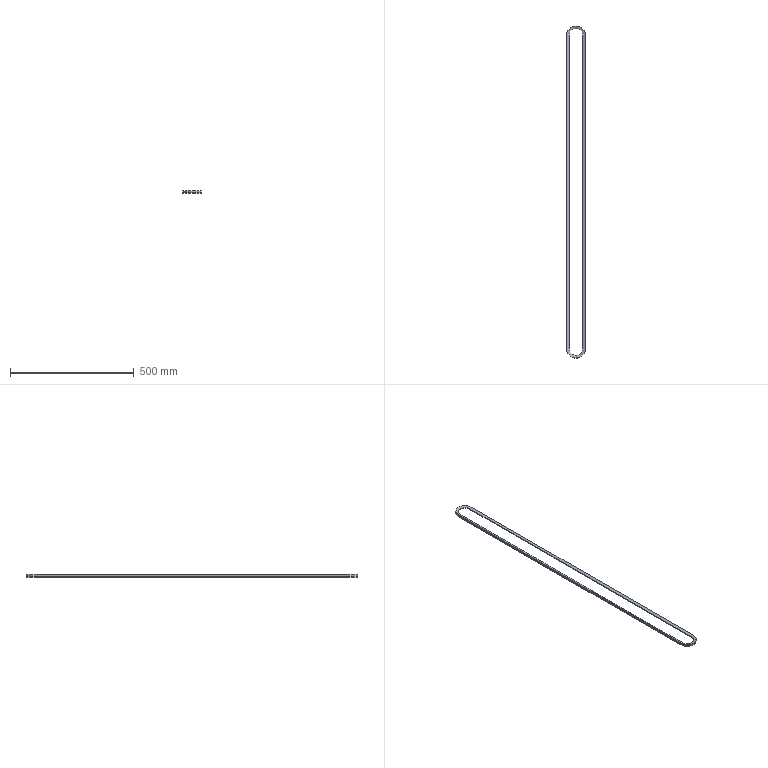Part | STEP file | 103000006124 | 1 solid | 24 faces | box 75 x 1341 x 10 mm | volume 174412 mm3 | plane 12 | cylinder 8 | cone 4 | commonest cylinder face diameters 55 x4 75 x4
STEP:
#1=CARTESIAN_POINT('',(27.5,-1266.,-1.36));
#2=VERTEX_POINT('',#1);
#3=CARTESIAN_POINT('',(37.5,-1266.,-5.));
#4=VERTEX_POINT('',#3);
#5=CARTESIAN_POINT('',(32.5,-1266.,-3.18));
#6=DIRECTION('',(0.9397,0.,-0.342));
#7=VECTOR('',#6,1.);
#8=LINE('',#5,#7);
#9=EDGE_CURVE('',#2,#4,#8,.T.);
#10=ORIENTED_EDGE('',*,*,#9,.F.);
#11=CARTESIAN_POINT('',(27.5,0.,-1.36));
#12=VERTEX_POINT('',#11);
#13=CARTESIAN_POINT('',(27.5,-633.,-1.36));
#14=DIRECTION('',(0.,1.,0.));
#15=VECTOR('',#14,1.);
#16=LINE('',#13,#15);
#17=EDGE_CURVE('',#2,#12,#16,.T.);
#18=ORIENTED_EDGE('',*,*,#17,.T.);
#19=CARTESIAN_POINT('',(37.5,0.,-5.));
#20=VERTEX_POINT('',#19);
#21=CARTESIAN_POINT('',(32.5,0.,-3.18));
#22=DIRECTION('',(0.9397,0.,-0.342));
#23=VECTOR('',#22,1.);
#24=LINE('',#21,#23);
#25=EDGE_CURVE('',#12,#20,#24,.T.);
#26=ORIENTED_EDGE('',*,*,#25,.T.);
#27=CARTESIAN_POINT('',(37.5,-633.,-5.));
#28=DIRECTION('',(0.,1.,0.));
#29=VECTOR('',#28,1.);
#30=LINE('',#27,#29);
#31=EDGE_CURVE('',#4,#20,#30,.T.);
#32=ORIENTED_EDGE('',*,*,#31,.F.);
#33=EDGE_LOOP('',(#10,#18,#26,#32));
#34=FACE_OUTER_BOUND('',#33,.T.);
#35=CARTESIAN_POINT('',(37.5,-1266.,-5.));
#36=DIRECTION('',(0.342,0.,0.9397));
#37=DIRECTION('',(0.9397,0.,-0.342));
#38=AXIS2_PLACEMENT_3D('',#35,#36,#37);
#39=PLANE('',#38);
#40=ADVANCED_FACE('',(#34),#39,.F.);
#41=CARTESIAN_POINT('',(-37.5,-1266.,-5.));
#42=VERTEX_POINT('',#41);
#43=CARTESIAN_POINT('',(0.,-1266.,-5.));
#44=DIRECTION('',(0.,0.,-1.));
#45=AXIS2_PLACEMENT_3D('',#43,#44,$);
#46=CIRCLE('',#45,37.5);
#47=EDGE_CURVE('',#42,#4,#46,.F.);
#48=ORIENTED_EDGE('',*,*,#47,.F.);
#49=CARTESIAN_POINT('',(-27.5,-1266.,-1.36));
#50=VERTEX_POINT('',#49);
#51=CARTESIAN_POINT('',(-469860.06,-1266.,-171006.427));
#52=DIRECTION('',(-0.9397,0.,-0.342));
#53=VECTOR('',#52,1.);
#54=LINE('',#51,#53);
#55=EDGE_CURVE('',#50,#42,#54,.T.);
#56=ORIENTED_EDGE('',*,*,#55,.F.);
#57=CARTESIAN_POINT('',(0.,-1266.,-1.36));
#58=DIRECTION('',(0.,0.,-1.));
#59=AXIS2_PLACEMENT_3D('',#57,#58,$);
#60=CIRCLE('',#59,27.5);
#61=EDGE_CURVE('',#50,#2,#60,.F.);
#62=ORIENTED_EDGE('',*,*,#61,.T.);
#63=ORIENTED_EDGE('',*,*,#9,.T.);
#64=EDGE_LOOP('',(#48,#56,#62,#63));
#65=FACE_OUTER_BOUND('',#64,.T.);
#66=CARTESIAN_POINT('',(0.,-1266.,-1.36));
#67=DIRECTION('',(0.,0.,-1.));
#68=DIRECTION('',(1.,0.,0.));
#69=AXIS2_PLACEMENT_3D('',#66,#67,#68);
#70=CONICAL_SURFACE('',#69,27.5,1.222);
#71=ADVANCED_FACE('',(#65),#70,.F.);
#72=CARTESIAN_POINT('',(27.5,-1266.,0.));
#73=VERTEX_POINT('',#72);
#74=CARTESIAN_POINT('',(27.5,0.,0.));
#75=VERTEX_POINT('',#74);
#76=CARTESIAN_POINT('',(27.5,-633.,0.));
#77=DIRECTION('',(0.,1.,0.));
#78=VECTOR('',#77,1.);
#79=LINE('',#76,#78);
#80=EDGE_CURVE('',#73,#75,#79,.T.);
#81=ORIENTED_EDGE('',*,*,#80,.T.);
#82=CARTESIAN_POINT('',(27.5,0.,-0.6801));
#83=DIRECTION('',(0.,0.,-1.));
#84=VECTOR('',#83,1.);
#85=LINE('',#82,#84);
#86=EDGE_CURVE('',#75,#12,#85,.T.);
#87=ORIENTED_EDGE('',*,*,#86,.T.);
#88=ORIENTED_EDGE('',*,*,#17,.F.);
#89=CARTESIAN_POINT('',(27.5,-1266.,-0.6801));
#90=DIRECTION('',(0.,0.,-1.));
#91=VECTOR('',#90,1.);
#92=LINE('',#89,#91);
#93=EDGE_CURVE('',#73,#2,#92,.T.);
#94=ORIENTED_EDGE('',*,*,#93,.F.);
#95=EDGE_LOOP('',(#81,#87,#88,#94));
#96=FACE_OUTER_BOUND('',#95,.T.);
#97=CARTESIAN_POINT('',(27.5,-1266.,0.));
#98=DIRECTION('',(1.,0.,0.));
#99=DIRECTION('',(0.,1.,0.));
#100=AXIS2_PLACEMENT_3D('',#97,#98,#99);
#101=PLANE('',#100);
#102=ADVANCED_FACE('',(#96),#101,.F.);
#103=CARTESIAN_POINT('',(-37.5,0.,-5.));
#104=VERTEX_POINT('',#103);
#105=CARTESIAN_POINT('',(0.,0.,-5.));
#106=DIRECTION('',(0.,0.,-1.));
#107=AXIS2_PLACEMENT_3D('',#105,#106,$);
#108=CIRCLE('',#107,37.5);
#109=EDGE_CURVE('',#20,#104,#108,.F.);
#110=ORIENTED_EDGE('',*,*,#109,.F.);
#111=ORIENTED_EDGE('',*,*,#25,.F.);
#112=CARTESIAN_POINT('',(-27.5,0.,-1.36));
#113=VERTEX_POINT('',#112);
#114=CARTESIAN_POINT('',(0.,0.,-1.36));
#115=DIRECTION('',(0.,0.,-1.));
#116=AXIS2_PLACEMENT_3D('',#114,#115,$);
#117=CIRCLE('',#116,27.5);
#118=EDGE_CURVE('',#12,#113,#117,.F.);
#119=ORIENTED_EDGE('',*,*,#118,.T.);
#120=CARTESIAN_POINT('',(-469860.06,0.,-171006.427));
#121=DIRECTION('',(-0.9397,0.,-0.342));
#122=VECTOR('',#121,1.);
#123=LINE('',#120,#122);
#124=EDGE_CURVE('',#113,#104,#123,.T.);
#125=ORIENTED_EDGE('',*,*,#124,.T.);
#126=EDGE_LOOP('',(#110,#111,#119,#125));
#127=FACE_OUTER_BOUND('',#126,.T.);
#128=CARTESIAN_POINT('',(0.,0.,-1.36));
#129=DIRECTION('',(0.,0.,-1.));
#130=DIRECTION('',(-1.,0.,0.));
#131=AXIS2_PLACEMENT_3D('',#128,#129,#130);
#132=CONICAL_SURFACE('',#131,27.5,1.222);
#133=ADVANCED_FACE('',(#127),#132,.F.);
#134=ORIENTED_EDGE('',*,*,#31,.T.);
#135=CARTESIAN_POINT('',(37.5,0.,0.));
#136=VERTEX_POINT('',#135);
#137=CARTESIAN_POINT('',(37.5,0.,-2.5));
#138=DIRECTION('',(0.,0.,1.));
#139=VECTOR('',#138,1.);
#140=LINE('',#137,#139);
#141=EDGE_CURVE('',#20,#136,#140,.T.);
#142=ORIENTED_EDGE('',*,*,#141,.T.);
#143=CARTESIAN_POINT('',(37.5,-1266.,0.));
#144=VERTEX_POINT('',#143);
#145=CARTESIAN_POINT('',(37.5,-633.,0.));
#146=DIRECTION('',(0.,1.,0.));
#147=VECTOR('',#146,1.);
#148=LINE('',#145,#147);
#149=EDGE_CURVE('',#144,#136,#148,.T.);
#150=ORIENTED_EDGE('',*,*,#149,.F.);
#151=CARTESIAN_POINT('',(37.5,-1266.,-2.5));
#152=DIRECTION('',(0.,0.,1.));
#153=VECTOR('',#152,1.);
#154=LINE('',#151,#153);
#155=EDGE_CURVE('',#4,#144,#154,.T.);
#156=ORIENTED_EDGE('',*,*,#155,.F.);
#157=EDGE_LOOP('',(#134,#142,#150,#156));
#158=FACE_OUTER_BOUND('',#157,.T.);
#159=CARTESIAN_POINT('',(37.5,-1266.,0.));
#160=DIRECTION('',(-1.,0.,0.));
#161=DIRECTION('',(0.,-1.,0.));
#162=AXIS2_PLACEMENT_3D('',#159,#160,#161);
#163=PLANE('',#162);
#164=ADVANCED_FACE('',(#158),#163,.F.);
#165=CARTESIAN_POINT('',(-37.5,-1266.,0.));
#166=VERTEX_POINT('',#165);
#167=CARTESIAN_POINT('',(0.,-1266.,0.));
#168=DIRECTION('',(0.,0.,1.));
#169=AXIS2_PLACEMENT_3D('',#167,#168,$);
#170=CIRCLE('',#169,37.5);
#171=EDGE_CURVE('',#166,#144,#170,.T.);
#172=ORIENTED_EDGE('',*,*,#171,.F.);
#173=CARTESIAN_POINT('',(-37.5,-1266.,0.));
#174=DIRECTION('',(0.,0.,1.));
#175=VECTOR('',#174,1.);
#176=LINE('',#173,#175);
#177=EDGE_CURVE('',#42,#166,#176,.T.);
#178=ORIENTED_EDGE('',*,*,#177,.F.);
#179=ORIENTED_EDGE('',*,*,#47,.T.);
#180=ORIENTED_EDGE('',*,*,#155,.T.);
#181=EDGE_LOOP('',(#172,#178,#179,#180));
#182=FACE_OUTER_BOUND('',#181,.T.);
#183=CARTESIAN_POINT('',(0.,-1266.,0.));
#184=DIRECTION('',(0.,0.,1.));
#185=DIRECTION('',(-1.,0.,0.));
#186=AXIS2_PLACEMENT_3D('',#183,#184,#185);
#187=CYLINDRICAL_SURFACE('',#186,37.5);
#188=ADVANCED_FACE('',(#182),#187,.T.);
#189=CARTESIAN_POINT('',(-37.5,-633.,-5.));
#190=DIRECTION('',(0.,-1.,0.));
#191=VECTOR('',#190,1.);
#192=LINE('',#189,#191);
#193=EDGE_CURVE('',#104,#42,#192,.T.);
#194=ORIENTED_EDGE('',*,*,#193,.F.);
#195=ORIENTED_EDGE('',*,*,#124,.F.);
#196=CARTESIAN_POINT('',(-27.5,-633.,-1.36));
#197=DIRECTION('',(0.,-1.,0.));
#198=VECTOR('',#197,1.);
#199=LINE('',#196,#198);
#200=EDGE_CURVE('',#113,#50,#199,.T.);
#201=ORIENTED_EDGE('',*,*,#200,.T.);
#202=ORIENTED_EDGE('',*,*,#55,.T.);
#203=EDGE_LOOP('',(#194,#195,#201,#202));
#204=FACE_OUTER_BOUND('',#203,.T.);
#205=CARTESIAN_POINT('',(-37.5,0.,-5.));
#206=DIRECTION('',(-0.342,0.,0.9397));
#207=DIRECTION('',(0.9397,0.,0.342));
#208=AXIS2_PLACEMENT_3D('',#205,#206,#207);
#209=PLANE('',#208);
#210=ADVANCED_FACE('',(#204),#209,.F.);
#211=ORIENTED_EDGE('',*,*,#93,.T.);
#212=ORIENTED_EDGE('',*,*,#61,.F.);
#213=CARTESIAN_POINT('',(-27.5,-1266.,0.));
#214=VERTEX_POINT('',#213);
#215=CARTESIAN_POINT('',(-27.5,-1266.,0.));
#216=DIRECTION('',(0.,0.,1.));
#217=VECTOR('',#216,1.);
#218=LINE('',#215,#217);
#219=EDGE_CURVE('',#214,#50,#218,.F.);
#220=ORIENTED_EDGE('',*,*,#219,.F.);
#221=CARTESIAN_POINT('',(0.,-1266.,0.));
#222=DIRECTION('',(0.,0.,1.));
#223=AXIS2_PLACEMENT_3D('',#221,#222,$);
#224=CIRCLE('',#223,27.5);
#225=EDGE_CURVE('',#214,#73,#224,.T.);
#226=ORIENTED_EDGE('',*,*,#225,.T.);
#227=EDGE_LOOP('',(#211,#212,#220,#226));
#228=FACE_OUTER_BOUND('',#227,.T.);
#229=CARTESIAN_POINT('',(0.,-1266.,0.));
#230=DIRECTION('',(0.,0.,1.));
#231=DIRECTION('',(-1.,0.,0.));
#232=AXIS2_PLACEMENT_3D('',#229,#230,#231);
#233=CYLINDRICAL_SURFACE('',#232,27.5);
#234=ADVANCED_FACE('',(#228),#233,.F.);
#235=CARTESIAN_POINT('',(27.5,-1266.,1.36));
#236=VERTEX_POINT('',#235);
#237=CARTESIAN_POINT('',(27.5,0.,1.36));
#238=VERTEX_POINT('',#237);
#239=CARTESIAN_POINT('',(27.5,-633.,1.36));
#240=DIRECTION('',(0.,1.,0.));
#241=VECTOR('',#240,1.);
#242=LINE('',#239,#241);
#243=EDGE_CURVE('',#236,#238,#242,.T.);
#244=ORIENTED_EDGE('',*,*,#243,.T.);
#245=CARTESIAN_POINT('',(27.5,0.,0.6801));
#246=DIRECTION('',(0.,0.,-1.));
#247=VECTOR('',#246,1.);
#248=LINE('',#245,#247);
#249=EDGE_CURVE('',#238,#75,#248,.T.);
#250=ORIENTED_EDGE('',*,*,#249,.T.);
#251=ORIENTED_EDGE('',*,*,#80,.F.);
#252=CARTESIAN_POINT('',(27.5,-1266.,0.6801));
#253=DIRECTION('',(0.,0.,-1.));
#254=VECTOR('',#253,1.);
#255=LINE('',#252,#254);
#256=EDGE_CURVE('',#236,#73,#255,.T.);
#257=ORIENTED_EDGE('',*,*,#256,.F.);
#258=EDGE_LOOP('',(#244,#250,#251,#257));
#259=FACE_OUTER_BOUND('',#258,.T.);
#260=CARTESIAN_POINT('',(27.5,-1266.,0.));
#261=DIRECTION('',(1.,0.,0.));
#262=DIRECTION('',(0.,1.,0.));
#263=AXIS2_PLACEMENT_3D('',#260,#261,#262);
#264=PLANE('',#263);
#265=ADVANCED_FACE('',(#259),#264,.F.);
#266=CARTESIAN_POINT('',(-27.5,0.,0.));
#267=VERTEX_POINT('',#266);
#268=CARTESIAN_POINT('',(-27.5,0.,0.));
#269=DIRECTION('',(0.,0.,1.));
#270=VECTOR('',#269,1.);
#271=LINE('',#268,#270);
#272=EDGE_CURVE('',#267,#113,#271,.F.);
#273=ORIENTED_EDGE('',*,*,#272,.T.);
#274=ORIENTED_EDGE('',*,*,#118,.F.);
#275=ORIENTED_EDGE('',*,*,#86,.F.);
#276=CARTESIAN_POINT('',(0.,0.,0.));
#277=DIRECTION('',(0.,0.,1.));
#278=AXIS2_PLACEMENT_3D('',#276,#277,$);
#279=CIRCLE('',#278,27.5);
#280=EDGE_CURVE('',#75,#267,#279,.T.);
#281=ORIENTED_EDGE('',*,*,#280,.T.);
#282=EDGE_LOOP('',(#273,#274,#275,#281));
#283=FACE_OUTER_BOUND('',#282,.T.);
#284=CARTESIAN_POINT('',(0.,0.,0.));
#285=DIRECTION('',(0.,0.,1.));
#286=DIRECTION('',(1.,0.,0.));
#287=AXIS2_PLACEMENT_3D('',#284,#285,#286);
#288=CYLINDRICAL_SURFACE('',#287,27.5);
#289=ADVANCED_FACE('',(#283),#288,.F.);
#290=CARTESIAN_POINT('',(-37.5,0.,0.));
#291=VERTEX_POINT('',#290);
#292=CARTESIAN_POINT('',(0.,0.,0.));
#293=DIRECTION('',(0.,0.,1.));
#294=AXIS2_PLACEMENT_3D('',#292,#293,$);
#295=CIRCLE('',#294,37.5);
#296=EDGE_CURVE('',#136,#291,#295,.T.);
#297=ORIENTED_EDGE('',*,*,#296,.F.);
#298=ORIENTED_EDGE('',*,*,#141,.F.);
#299=ORIENTED_EDGE('',*,*,#109,.T.);
#300=CARTESIAN_POINT('',(-37.5,0.,0.));
#301=DIRECTION('',(0.,0.,1.));
#302=VECTOR('',#301,1.);
#303=LINE('',#300,#302);
#304=EDGE_CURVE('',#104,#291,#303,.T.);
#305=ORIENTED_EDGE('',*,*,#304,.T.);
#306=EDGE_LOOP('',(#297,#298,#299,#305));
#307=FACE_OUTER_BOUND('',#306,.T.);
#308=CARTESIAN_POINT('',(0.,0.,0.));
#309=DIRECTION('',(0.,0.,1.));
#310=DIRECTION('',(1.,0.,0.));
#311=AXIS2_PLACEMENT_3D('',#308,#309,#310);
#312=CYLINDRICAL_SURFACE('',#311,37.5);
#313=ADVANCED_FACE('',(#307),#312,.T.);
#314=ORIENTED_EDGE('',*,*,#149,.T.);
#315=CARTESIAN_POINT('',(37.5,0.,5.));
#316=VERTEX_POINT('',#315);
#317=CARTESIAN_POINT('',(37.5,0.,2.5));
#318=DIRECTION('',(0.,0.,1.));
#319=VECTOR('',#318,1.);
#320=LINE('',#317,#319);
#321=EDGE_CURVE('',#136,#316,#320,.T.);
#322=ORIENTED_EDGE('',*,*,#321,.T.);
#323=CARTESIAN_POINT('',(37.5,-1266.,5.));
#324=VERTEX_POINT('',#323);
#325=CARTESIAN_POINT('',(37.5,-633.,5.));
#326=DIRECTION('',(0.,1.,0.));
#327=VECTOR('',#326,1.);
#328=LINE('',#325,#327);
#329=EDGE_CURVE('',#324,#316,#328,.T.);
#330=ORIENTED_EDGE('',*,*,#329,.F.);
#331=CARTESIAN_POINT('',(37.5,-1266.,2.5));
#332=DIRECTION('',(0.,0.,1.));
#333=VECTOR('',#332,1.);
#334=LINE('',#331,#333);
#335=EDGE_CURVE('',#144,#324,#334,.T.);
#336=ORIENTED_EDGE('',*,*,#335,.F.);
#337=EDGE_LOOP('',(#314,#322,#330,#336));
#338=FACE_OUTER_BOUND('',#337,.T.);
#339=CARTESIAN_POINT('',(37.5,-1266.,0.));
#340=DIRECTION('',(-1.,0.,0.));
#341=DIRECTION('',(0.,-1.,0.));
#342=AXIS2_PLACEMENT_3D('',#339,#340,#341);
#343=PLANE('',#342);
#344=ADVANCED_FACE('',(#338),#343,.F.);
#345=CARTESIAN_POINT('',(-37.5,-1266.,5.));
#346=VERTEX_POINT('',#345);
#347=CARTESIAN_POINT('',(0.,-1266.,5.));
#348=DIRECTION('',(0.,0.,1.));
#349=AXIS2_PLACEMENT_3D('',#347,#348,$);
#350=CIRCLE('',#349,37.5);
#351=EDGE_CURVE('',#346,#324,#350,.T.);
#352=ORIENTED_EDGE('',*,*,#351,.F.);
#353=CARTESIAN_POINT('',(-37.5,-1266.,0.));
#354=DIRECTION('',(0.,0.,1.));
#355=VECTOR('',#354,1.);
#356=LINE('',#353,#355);
#357=EDGE_CURVE('',#166,#346,#356,.T.);
#358=ORIENTED_EDGE('',*,*,#357,.F.);
#359=ORIENTED_EDGE('',*,*,#171,.T.);
#360=ORIENTED_EDGE('',*,*,#335,.T.);
#361=EDGE_LOOP('',(#352,#358,#359,#360));
#362=FACE_OUTER_BOUND('',#361,.T.);
#363=CARTESIAN_POINT('',(0.,-1266.,0.));
#364=DIRECTION('',(0.,0.,1.));
#365=DIRECTION('',(-1.,0.,0.));
#366=AXIS2_PLACEMENT_3D('',#363,#364,#365);
#367=CYLINDRICAL_SURFACE('',#366,37.5);
#368=ADVANCED_FACE('',(#362),#367,.T.);
#369=CARTESIAN_POINT('',(-37.5,-633.,0.));
#370=DIRECTION('',(0.,-1.,0.));
#371=VECTOR('',#370,1.);
#372=LINE('',#369,#371);
#373=EDGE_CURVE('',#291,#166,#372,.T.);
#374=ORIENTED_EDGE('',*,*,#373,.F.);
#375=ORIENTED_EDGE('',*,*,#304,.F.);
#376=ORIENTED_EDGE('',*,*,#193,.T.);
#377=ORIENTED_EDGE('',*,*,#177,.T.);
#378=EDGE_LOOP('',(#374,#375,#376,#377));
#379=FACE_OUTER_BOUND('',#378,.T.);
#380=CARTESIAN_POINT('',(-37.5,0.,0.));
#381=DIRECTION('',(1.,0.,0.));
#382=DIRECTION('',(0.,1.,0.));
#383=AXIS2_PLACEMENT_3D('',#380,#381,#382);
#384=PLANE('',#383);
#385=ADVANCED_FACE('',(#379),#384,.F.);
#386=ORIENTED_EDGE('',*,*,#219,.T.);
#387=ORIENTED_EDGE('',*,*,#200,.F.);
#388=ORIENTED_EDGE('',*,*,#272,.F.);
#389=CARTESIAN_POINT('',(-27.5,-633.,0.));
#390=DIRECTION('',(0.,-1.,0.));
#391=VECTOR('',#390,1.);
#392=LINE('',#389,#391);
#393=EDGE_CURVE('',#267,#214,#392,.T.);
#394=ORIENTED_EDGE('',*,*,#393,.T.);
#395=EDGE_LOOP('',(#386,#387,#388,#394));
#396=FACE_OUTER_BOUND('',#395,.T.);
#397=CARTESIAN_POINT('',(-27.5,0.,0.));
#398=DIRECTION('',(-1.,0.,0.));
#399=DIRECTION('',(0.,-1.,0.));
#400=AXIS2_PLACEMENT_3D('',#397,#398,#399);
#401=PLANE('',#400);
#402=ADVANCED_FACE('',(#396),#401,.F.);
#403=ORIENTED_EDGE('',*,*,#225,.F.);
#404=CARTESIAN_POINT('',(-27.5,-1266.,1.36));
#405=VERTEX_POINT('',#404);
#406=CARTESIAN_POINT('',(-27.5,-1266.,0.));
#407=DIRECTION('',(0.,0.,1.));
#408=VECTOR('',#407,1.);
#409=LINE('',#406,#408);
#410=EDGE_CURVE('',#405,#214,#409,.F.);
#411=ORIENTED_EDGE('',*,*,#410,.F.);
#412=CARTESIAN_POINT('',(-27.5,-1266.,1.36));
#413=CARTESIAN_POINT('',(-27.5,-1270.32,1.36));
#414=CARTESIAN_POINT('',(-26.652,-1274.639,1.36));
#415=CARTESIAN_POINT('',(-24.955,-1278.737,1.36));
#416=CARTESIAN_POINT('',(-20.045,-1286.045,1.36));
#417=CARTESIAN_POINT('',(-12.737,-1290.955,1.36));
#418=CARTESIAN_POINT('',(-8.639,-1292.652,1.36));
#419=CARTESIAN_POINT('',(0.,-1294.348,1.36));
#420=CARTESIAN_POINT('',(8.639,-1292.652,1.36));
#421=CARTESIAN_POINT('',(12.737,-1290.955,1.36));
#422=CARTESIAN_POINT('',(20.045,-1286.045,1.36));
#423=CARTESIAN_POINT('',(24.955,-1278.737,1.36));
#424=CARTESIAN_POINT('',(26.652,-1274.639,1.36));
#425=CARTESIAN_POINT('',(27.5,-1270.32,1.36));
#426=CARTESIAN_POINT('',(27.5,-1266.,1.36));
#427=B_SPLINE_CURVE_WITH_KNOTS('',5,(#412,#413,#414,#415,#416,#417,#418,#419,#420,#421,#422,#423,#424,#425,#426),.UNSPECIFIED.,.F.,.U.,(6,3,3,3,6),(-43.197,-21.598,0.,21.598,43.197),.UNSPECIFIED.);
#428=EDGE_CURVE('',#405,#236,#427,.T.);
#429=ORIENTED_EDGE('',*,*,#428,.T.);
#430=ORIENTED_EDGE('',*,*,#256,.T.);
#431=EDGE_LOOP('',(#403,#411,#429,#430));
#432=FACE_OUTER_BOUND('',#431,.T.);
#433=CARTESIAN_POINT('',(0.,-1266.,0.));
#434=DIRECTION('',(0.,0.,1.));
#435=DIRECTION('',(-1.,0.,0.));
#436=AXIS2_PLACEMENT_3D('',#433,#434,#435);
#437=CYLINDRICAL_SURFACE('',#436,27.5);
#438=ADVANCED_FACE('',(#432),#437,.F.);
#439=ORIENTED_EDGE('',*,*,#329,.T.);
#440=CARTESIAN_POINT('',(32.5,0.,3.18));
#441=DIRECTION('',(-0.9397,0.,-0.342));
#442=VECTOR('',#441,1.);
#443=LINE('',#440,#442);
#444=EDGE_CURVE('',#316,#238,#443,.T.);
#445=ORIENTED_EDGE('',*,*,#444,.T.);
#446=ORIENTED_EDGE('',*,*,#243,.F.);
#447=CARTESIAN_POINT('',(32.5,-1266.,3.18));
#448=DIRECTION('',(-0.9397,0.,-0.342));
#449=VECTOR('',#448,1.);
#450=LINE('',#447,#449);
#451=EDGE_CURVE('',#324,#236,#450,.T.);
#452=ORIENTED_EDGE('',*,*,#451,.F.);
#453=EDGE_LOOP('',(#439,#445,#446,#452));
#454=FACE_OUTER_BOUND('',#453,.T.);
#455=CARTESIAN_POINT('',(37.5,-1266.,5.));
#456=DIRECTION('',(0.342,0.,-0.9397));
#457=DIRECTION('',(-0.9397,0.,-0.342));
#458=AXIS2_PLACEMENT_3D('',#455,#456,#457);
#459=PLANE('',#458);
#460=ADVANCED_FACE('',(#454),#459,.F.);
#461=ORIENTED_EDGE('',*,*,#280,.F.);
#462=ORIENTED_EDGE('',*,*,#249,.F.);
#463=CARTESIAN_POINT('',(-27.5,0.,1.36));
#464=VERTEX_POINT('',#463);
#465=CARTESIAN_POINT('',(0.,0.,1.36));
#466=DIRECTION('',(0.,0.,1.));
#467=AXIS2_PLACEMENT_3D('',#465,#466,$);
#468=CIRCLE('',#467,27.5);
#469=EDGE_CURVE('',#238,#464,#468,.T.);
#470=ORIENTED_EDGE('',*,*,#469,.T.);
#471=CARTESIAN_POINT('',(-27.5,0.,0.));
#472=DIRECTION('',(0.,0.,1.));
#473=VECTOR('',#472,1.);
#474=LINE('',#471,#473);
#475=EDGE_CURVE('',#464,#267,#474,.F.);
#476=ORIENTED_EDGE('',*,*,#475,.T.);
#477=EDGE_LOOP('',(#461,#462,#470,#476));
#478=FACE_OUTER_BOUND('',#477,.T.);
#479=CARTESIAN_POINT('',(0.,0.,0.));
#480=DIRECTION('',(0.,0.,1.));
#481=DIRECTION('',(1.,0.,0.));
#482=AXIS2_PLACEMENT_3D('',#479,#480,#481);
#483=CYLINDRICAL_SURFACE('',#482,27.5);
#484=ADVANCED_FACE('',(#478),#483,.F.);
#485=CARTESIAN_POINT('',(-37.5,0.,5.));
#486=VERTEX_POINT('',#485);
#487=CARTESIAN_POINT('',(0.,0.,5.));
#488=DIRECTION('',(0.,0.,1.));
#489=AXIS2_PLACEMENT_3D('',#487,#488,$);
#490=CIRCLE('',#489,37.5);
#491=EDGE_CURVE('',#316,#486,#490,.T.);
#492=ORIENTED_EDGE('',*,*,#491,.F.);
#493=ORIENTED_EDGE('',*,*,#321,.F.);
#494=ORIENTED_EDGE('',*,*,#296,.T.);
#495=CARTESIAN_POINT('',(-37.5,0.,0.));
#496=DIRECTION('',(0.,0.,1.));
#497=VECTOR('',#496,1.);
#498=LINE('',#495,#497);
#499=EDGE_CURVE('',#291,#486,#498,.T.);
#500=ORIENTED_EDGE('',*,*,#499,.T.);
#501=EDGE_LOOP('',(#492,#493,#494,#500));
#502=FACE_OUTER_BOUND('',#501,.T.);
#503=CARTESIAN_POINT('',(0.,0.,0.));
#504=DIRECTION('',(0.,0.,1.));
#505=DIRECTION('',(1.,0.,0.));
#506=AXIS2_PLACEMENT_3D('',#503,#504,#505);
#507=CYLINDRICAL_SURFACE('',#506,37.5);
#508=ADVANCED_FACE('',(#502),#507,.T.);
#509=ORIENTED_EDGE('',*,*,#428,.F.);
#510=CARTESIAN_POINT('',(-469865.06,-1266.,171008.247));
#511=DIRECTION('',(-0.9397,0.,0.342));
#512=VECTOR('',#511,1.);
#513=LINE('',#510,#512);
#514=EDGE_CURVE('',#346,#405,#513,.F.);
#515=ORIENTED_EDGE('',*,*,#514,.F.);
#516=ORIENTED_EDGE('',*,*,#351,.T.);
#517=ORIENTED_EDGE('',*,*,#451,.T.);
#518=EDGE_LOOP('',(#509,#515,#516,#517));
#519=FACE_OUTER_BOUND('',#518,.T.);
#520=CARTESIAN_POINT('',(0.,-1266.,5.));
#521=DIRECTION('',(0.,0.,1.));
#522=DIRECTION('',(-1.,0.,0.));
#523=AXIS2_PLACEMENT_3D('',#520,#521,#522);
#524=CONICAL_SURFACE('',#523,37.5,1.222);
#525=ADVANCED_FACE('',(#519),#524,.F.);
#526=CARTESIAN_POINT('',(-37.5,-633.,5.));
#527=DIRECTION('',(0.,-1.,0.));
#528=VECTOR('',#527,1.);
#529=LINE('',#526,#528);
#530=EDGE_CURVE('',#486,#346,#529,.T.);
#531=ORIENTED_EDGE('',*,*,#530,.F.);
#532=ORIENTED_EDGE('',*,*,#499,.F.);
#533=ORIENTED_EDGE('',*,*,#373,.T.);
#534=ORIENTED_EDGE('',*,*,#357,.T.);
#535=EDGE_LOOP('',(#531,#532,#533,#534));
#536=FACE_OUTER_BOUND('',#535,.T.);
#537=CARTESIAN_POINT('',(-37.5,0.,0.));
#538=DIRECTION('',(1.,0.,0.));
#539=DIRECTION('',(0.,1.,0.));
#540=AXIS2_PLACEMENT_3D('',#537,#538,#539);
#541=PLANE('',#540);
#542=ADVANCED_FACE('',(#536),#541,.F.);
#543=ORIENTED_EDGE('',*,*,#393,.F.);
#544=ORIENTED_EDGE('',*,*,#475,.F.);
#545=CARTESIAN_POINT('',(-27.5,-633.,1.36));
#546=DIRECTION('',(0.,-1.,0.));
#547=VECTOR('',#546,1.);
#548=LINE('',#545,#547);
#549=EDGE_CURVE('',#464,#405,#548,.T.);
#550=ORIENTED_EDGE('',*,*,#549,.T.);
#551=ORIENTED_EDGE('',*,*,#410,.T.);
#552=EDGE_LOOP('',(#543,#544,#550,#551));
#553=FACE_OUTER_BOUND('',#552,.T.);
#554=CARTESIAN_POINT('',(-27.5,0.,0.));
#555=DIRECTION('',(-1.,0.,0.));
#556=DIRECTION('',(0.,-1.,0.));
#557=AXIS2_PLACEMENT_3D('',#554,#555,#556);
#558=PLANE('',#557);
#559=ADVANCED_FACE('',(#553),#558,.F.);
#560=ORIENTED_EDGE('',*,*,#469,.F.);
#561=ORIENTED_EDGE('',*,*,#444,.F.);
#562=ORIENTED_EDGE('',*,*,#491,.T.);
#563=CARTESIAN_POINT('',(-469865.06,0.,171008.247));
#564=DIRECTION('',(-0.9397,0.,0.342));
#565=VECTOR('',#564,1.);
#566=LINE('',#563,#565);
#567=EDGE_CURVE('',#486,#464,#566,.F.);
#568=ORIENTED_EDGE('',*,*,#567,.T.);
#569=EDGE_LOOP('',(#560,#561,#562,#568));
#570=FACE_OUTER_BOUND('',#569,.T.);
#571=CARTESIAN_POINT('',(0.,0.,5.));
#572=DIRECTION('',(0.,0.,1.));
#573=DIRECTION('',(1.,0.,0.));
#574=AXIS2_PLACEMENT_3D('',#571,#572,#573);
#575=CONICAL_SURFACE('',#574,37.5,1.222);
#576=ADVANCED_FACE('',(#570),#575,.F.);
#577=ORIENTED_EDGE('',*,*,#549,.F.);
#578=ORIENTED_EDGE('',*,*,#567,.F.);
#579=ORIENTED_EDGE('',*,*,#530,.T.);
#580=ORIENTED_EDGE('',*,*,#514,.T.);
#581=EDGE_LOOP('',(#577,#578,#579,#580));
#582=FACE_OUTER_BOUND('',#581,.T.);
#583=CARTESIAN_POINT('',(-37.5,0.,5.));
#584=DIRECTION('',(-0.342,0.,-0.9397));
#585=DIRECTION('',(-0.9397,0.,0.342));
#586=AXIS2_PLACEMENT_3D('',#583,#584,#585);
#587=PLANE('',#586);
#588=ADVANCED_FACE('',(#582),#587,.F.);
#589=CLOSED_SHELL('',(#40,#71,#102,#133,#164,#188,#210,#234,#265,#289,#313,#344,#368,#385,#402,#438,#460,#484,#508,#525,#542,#559,#576,#588));
#590=MANIFOLD_SOLID_BREP('',#589);
#591=(LENGTH_UNIT()NAMED_UNIT(*)SI_UNIT(.MILLI.,.METRE.));
#592=UNCERTAINTY_MEASURE_WITH_UNIT(LENGTH_MEASURE(0.005),#591,'','');
#593=(NAMED_UNIT(*)PLANE_ANGLE_UNIT()SI_UNIT($,.RADIAN.));
#594=(NAMED_UNIT(*)SI_UNIT($,.STERADIAN.)SOLID_ANGLE_UNIT());
#595=(GEOMETRIC_REPRESENTATION_CONTEXT(3)GLOBAL_UNCERTAINTY_ASSIGNED_CONTEXT((#592))GLOBAL_UNIT_ASSIGNED_CONTEXT((#591,#593,#594))REPRESENTATION_CONTEXT('',''));
#596=ADVANCED_BREP_SHAPE_REPRESENTATION('',(#590),#595);